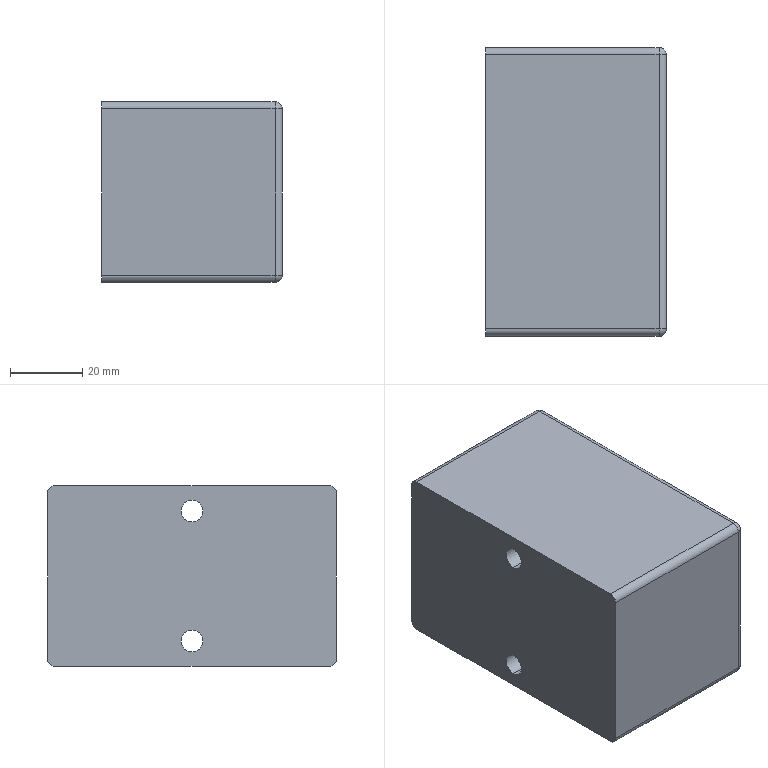Part | STEP file | 4-20.sldasm-Part-101 | 1 solid | 28 faces | box 50 x 80 x 50 mm | volume 195848 mm3 | cylinder 16 | plane 8 | sphere 4 | commonest cylinder face diameters 4 x8 6 x4 11 x4
STEP:
#1=CARTESIAN_POINT('',(268.,-172.617,-89.093));
#2=VERTEX_POINT('',#1);
#3=CARTESIAN_POINT('',(268.,-172.617,-78.093));
#4=VERTEX_POINT('',#3);
#5=CARTESIAN_POINT('',(268.,-172.617,-83.593));
#6=DIRECTION('',(1.,0.,0.));
#7=DIRECTION('',(0.,0.,-1.));
#8=AXIS2_PLACEMENT_3D('',#5,#6,#7);
#9=CIRCLE('',#8,5.5);
#10=EDGE_CURVE('',#2,#4,#9,.T.);
#11=ORIENTED_EDGE('',*,*,#10,.F.);
#12=CARTESIAN_POINT('',(274.936,-172.617,-89.093));
#13=VERTEX_POINT('',#12);
#14=CARTESIAN_POINT('',(268.,-172.617,-89.093));
#15=DIRECTION('',(1.,0.,0.));
#16=VECTOR('',#15,1000.);
#17=LINE('',#14,#16);
#18=EDGE_CURVE('',#2,#13,#17,.T.);
#19=ORIENTED_EDGE('',*,*,#18,.T.);
#20=CARTESIAN_POINT('',(275.,-170.326,-88.593));
#21=VERTEX_POINT('',#20);
#22=CARTESIAN_POINT('',(274.936,-172.617,-89.093));
#23=CARTESIAN_POINT('',(274.936,-172.225,-89.093));
#24=CARTESIAN_POINT('',(274.949,-171.836,-89.052));
#25=CARTESIAN_POINT('',(274.981,-171.063,-88.884));
#26=CARTESIAN_POINT('',(275.,-170.687,-88.758));
#27=CARTESIAN_POINT('',(275.,-170.326,-88.593));
#28=B_SPLINE_CURVE_WITH_KNOTS('',3,(#22,#23,#24,#25,#26,#27),.UNSPECIFIED.,.F.,.F.,(4,2,4),(0.002353,0.003528,0.004703),.UNSPECIFIED.);
#29=EDGE_CURVE('',#13,#21,#28,.T.);
#30=ORIENTED_EDGE('',*,*,#29,.T.);
#31=CARTESIAN_POINT('',(275.,-172.617,-78.093));
#32=VERTEX_POINT('',#31);
#33=CARTESIAN_POINT('',(275.,-172.617,-83.593));
#34=DIRECTION('',(1.,0.,0.));
#35=DIRECTION('',(0.,0.,-1.));
#36=AXIS2_PLACEMENT_3D('',#33,#34,#35);
#37=CIRCLE('',#36,5.5);
#38=EDGE_CURVE('',#21,#32,#37,.T.);
#39=ORIENTED_EDGE('',*,*,#38,.T.);
#40=CARTESIAN_POINT('',(268.,-172.617,-78.093));
#41=DIRECTION('',(1.,0.,0.));
#42=VECTOR('',#41,1000.);
#43=LINE('',#40,#42);
#44=EDGE_CURVE('',#4,#32,#43,.T.);
#45=ORIENTED_EDGE('',*,*,#44,.F.);
#46=EDGE_LOOP('',(#11,#19,#30,#39,#45));
#47=FACE_OUTER_BOUND('',#46,.T.);
#48=CARTESIAN_POINT('',(268.,-172.617,-83.593));
#49=DIRECTION('',(1.,0.,0.));
#50=DIRECTION('',(0.,0.,1.));
#51=AXIS2_PLACEMENT_3D('',#48,#49,#50);
#52=CYLINDRICAL_SURFACE('',#51,5.5);
#53=ADVANCED_FACE('',(#47),#52,.F.);
#54=CARTESIAN_POINT('',(268.,-172.617,-86.593));
#55=VERTEX_POINT('',#54);
#56=CARTESIAN_POINT('',(268.,-172.617,-80.593));
#57=VERTEX_POINT('',#56);
#58=CARTESIAN_POINT('',(268.,-172.617,-83.593));
#59=DIRECTION('',(1.,0.,0.));
#60=DIRECTION('',(0.,0.,-1.));
#61=AXIS2_PLACEMENT_3D('',#58,#59,#60);
#62=CIRCLE('',#61,3.);
#63=EDGE_CURVE('',#55,#57,#62,.T.);
#64=ORIENTED_EDGE('',*,*,#63,.T.);
#65=CARTESIAN_POINT('',(225.,-172.617,-80.593));
#66=VERTEX_POINT('',#65);
#67=CARTESIAN_POINT('',(232.,-172.617,-80.593));
#68=DIRECTION('',(-1.,0.,0.));
#69=VECTOR('',#68,1000.);
#70=LINE('',#67,#69);
#71=EDGE_CURVE('',#57,#66,#70,.T.);
#72=ORIENTED_EDGE('',*,*,#71,.T.);
#73=CARTESIAN_POINT('',(225.,-172.617,-86.593));
#74=VERTEX_POINT('',#73);
#75=CARTESIAN_POINT('',(225.,-172.617,-83.593));
#76=DIRECTION('',(1.,0.,0.));
#77=DIRECTION('',(0.,0.,1.));
#78=AXIS2_PLACEMENT_3D('',#75,#76,#77);
#79=CIRCLE('',#78,3.);
#80=EDGE_CURVE('',#74,#66,#79,.T.);
#81=ORIENTED_EDGE('',*,*,#80,.F.);
#82=CARTESIAN_POINT('',(232.,-172.617,-86.593));
#83=DIRECTION('',(-1.,0.,0.));
#84=VECTOR('',#83,1000.);
#85=LINE('',#82,#84);
#86=EDGE_CURVE('',#55,#74,#85,.T.);
#87=ORIENTED_EDGE('',*,*,#86,.F.);
#88=EDGE_LOOP('',(#64,#72,#81,#87));
#89=FACE_OUTER_BOUND('',#88,.T.);
#90=CARTESIAN_POINT('',(232.,-172.617,-83.593));
#91=DIRECTION('',(-1.,0.,0.));
#92=DIRECTION('',(0.,0.,-1.));
#93=AXIS2_PLACEMENT_3D('',#90,#91,#92);
#94=CYLINDRICAL_SURFACE('',#93,3.);
#95=ADVANCED_FACE('',(#89),#94,.F.);
#96=CARTESIAN_POINT('',(268.,-172.617,-53.093));
#97=VERTEX_POINT('',#96);
#98=CARTESIAN_POINT('',(268.,-172.617,-42.093));
#99=VERTEX_POINT('',#98);
#100=CARTESIAN_POINT('',(268.,-172.617,-47.593));
#101=DIRECTION('',(-1.,0.,0.));
#102=DIRECTION('',(0.,0.,1.));
#103=AXIS2_PLACEMENT_3D('',#100,#101,#102);
#104=CIRCLE('',#103,5.5);
#105=EDGE_CURVE('',#97,#99,#104,.T.);
#106=ORIENTED_EDGE('',*,*,#105,.T.);
#107=CARTESIAN_POINT('',(274.936,-172.617,-42.093));
#108=VERTEX_POINT('',#107);
#109=CARTESIAN_POINT('',(268.,-172.617,-42.093));
#110=DIRECTION('',(1.,0.,0.));
#111=VECTOR('',#110,1000.);
#112=LINE('',#109,#111);
#113=EDGE_CURVE('',#99,#108,#112,.T.);
#114=ORIENTED_EDGE('',*,*,#113,.T.);
#115=CARTESIAN_POINT('',(275.,-174.908,-42.593));
#116=VERTEX_POINT('',#115);
#117=CARTESIAN_POINT('',(274.936,-172.617,-42.093));
#118=CARTESIAN_POINT('',(274.936,-173.009,-42.093));
#119=CARTESIAN_POINT('',(274.949,-173.398,-42.134));
#120=CARTESIAN_POINT('',(274.981,-174.171,-42.302));
#121=CARTESIAN_POINT('',(275.,-174.547,-42.428));
#122=CARTESIAN_POINT('',(275.,-174.908,-42.593));
#123=B_SPLINE_CURVE_WITH_KNOTS('',3,(#117,#118,#119,#120,#121,#122),.UNSPECIFIED.,.F.,.F.,(4,2,4),(0.002353,0.003528,0.004703),.UNSPECIFIED.);
#124=EDGE_CURVE('',#108,#116,#123,.T.);
#125=ORIENTED_EDGE('',*,*,#124,.T.);
#126=CARTESIAN_POINT('',(275.,-172.617,-53.093));
#127=VERTEX_POINT('',#126);
#128=CARTESIAN_POINT('',(275.,-172.617,-47.593));
#129=DIRECTION('',(1.,0.,0.));
#130=DIRECTION('',(0.,0.,-1.));
#131=AXIS2_PLACEMENT_3D('',#128,#129,#130);
#132=CIRCLE('',#131,5.5);
#133=EDGE_CURVE('',#116,#127,#132,.T.);
#134=ORIENTED_EDGE('',*,*,#133,.T.);
#135=CARTESIAN_POINT('',(268.,-172.617,-53.093));
#136=DIRECTION('',(1.,0.,0.));
#137=VECTOR('',#136,1000.);
#138=LINE('',#135,#137);
#139=EDGE_CURVE('',#97,#127,#138,.T.);
#140=ORIENTED_EDGE('',*,*,#139,.F.);
#141=EDGE_LOOP('',(#106,#114,#125,#134,#140));
#142=FACE_OUTER_BOUND('',#141,.T.);
#143=CARTESIAN_POINT('',(268.,-172.617,-47.593));
#144=DIRECTION('',(1.,0.,0.));
#145=DIRECTION('',(0.,0.,-1.));
#146=AXIS2_PLACEMENT_3D('',#143,#144,#145);
#147=CYLINDRICAL_SURFACE('',#146,5.5);
#148=ADVANCED_FACE('',(#142),#147,.F.);
#149=CARTESIAN_POINT('',(268.,-172.617,-50.593));
#150=VERTEX_POINT('',#149);
#151=CARTESIAN_POINT('',(268.,-172.617,-44.593));
#152=VERTEX_POINT('',#151);
#153=CARTESIAN_POINT('',(268.,-172.617,-47.593));
#154=DIRECTION('',(-1.,0.,0.));
#155=DIRECTION('',(0.,0.,1.));
#156=AXIS2_PLACEMENT_3D('',#153,#154,#155);
#157=CIRCLE('',#156,3.);
#158=EDGE_CURVE('',#150,#152,#157,.T.);
#159=ORIENTED_EDGE('',*,*,#158,.F.);
#160=CARTESIAN_POINT('',(225.,-172.617,-50.593));
#161=VERTEX_POINT('',#160);
#162=CARTESIAN_POINT('',(232.,-172.617,-50.593));
#163=DIRECTION('',(-1.,0.,0.));
#164=VECTOR('',#163,1000.);
#165=LINE('',#162,#164);
#166=EDGE_CURVE('',#150,#161,#165,.T.);
#167=ORIENTED_EDGE('',*,*,#166,.T.);
#168=CARTESIAN_POINT('',(225.,-172.617,-44.593));
#169=VERTEX_POINT('',#168);
#170=CARTESIAN_POINT('',(225.,-172.617,-47.593));
#171=DIRECTION('',(1.,0.,0.));
#172=DIRECTION('',(0.,0.,1.));
#173=AXIS2_PLACEMENT_3D('',#170,#171,#172);
#174=CIRCLE('',#173,3.);
#175=EDGE_CURVE('',#169,#161,#174,.T.);
#176=ORIENTED_EDGE('',*,*,#175,.F.);
#177=CARTESIAN_POINT('',(232.,-172.617,-44.593));
#178=DIRECTION('',(-1.,0.,0.));
#179=VECTOR('',#178,1000.);
#180=LINE('',#177,#179);
#181=EDGE_CURVE('',#152,#169,#180,.T.);
#182=ORIENTED_EDGE('',*,*,#181,.F.);
#183=EDGE_LOOP('',(#159,#167,#176,#182));
#184=FACE_OUTER_BOUND('',#183,.T.);
#185=CARTESIAN_POINT('',(232.,-172.617,-47.593));
#186=DIRECTION('',(-1.,0.,0.));
#187=DIRECTION('',(0.,0.,1.));
#188=AXIS2_PLACEMENT_3D('',#185,#186,#187);
#189=CYLINDRICAL_SURFACE('',#188,3.);
#190=ADVANCED_FACE('',(#184),#189,.F.);
#191=ORIENTED_EDGE('',*,*,#175,.T.);
#192=CARTESIAN_POINT('',(225.,-172.617,-47.593));
#193=DIRECTION('',(1.,0.,0.));
#194=DIRECTION('',(0.,0.,1.));
#195=AXIS2_PLACEMENT_3D('',#192,#193,#194);
#196=CIRCLE('',#195,3.);
#197=EDGE_CURVE('',#161,#169,#196,.T.);
#198=ORIENTED_EDGE('',*,*,#197,.T.);
#199=EDGE_LOOP('',(#191,#198));
#200=FACE_BOUND('',#199,.T.);
#201=CARTESIAN_POINT('',(225.,-134.617,-90.593));
#202=VERTEX_POINT('',#201);
#203=CARTESIAN_POINT('',(225.,-210.617,-90.593));
#204=VERTEX_POINT('',#203);
#205=CARTESIAN_POINT('',(225.,-112.617,-90.593));
#206=DIRECTION('',(0.,-1.,0.));
#207=VECTOR('',#206,1000.);
#208=LINE('',#205,#207);
#209=EDGE_CURVE('',#202,#204,#208,.T.);
#210=ORIENTED_EDGE('',*,*,#209,.T.);
#211=CARTESIAN_POINT('',(225.,-212.617,-88.593));
#212=VERTEX_POINT('',#211);
#213=CARTESIAN_POINT('',(225.,-210.617,-88.593));
#214=DIRECTION('',(-1.,0.,0.));
#215=DIRECTION('',(0.,0.,1.));
#216=AXIS2_PLACEMENT_3D('',#213,#214,#215);
#217=CIRCLE('',#216,2.);
#218=EDGE_CURVE('',#204,#212,#217,.T.);
#219=ORIENTED_EDGE('',*,*,#218,.T.);
#220=CARTESIAN_POINT('',(225.,-212.617,-42.593));
#221=VERTEX_POINT('',#220);
#222=CARTESIAN_POINT('',(225.,-212.617,-65.593));
#223=DIRECTION('',(0.,0.,1.));
#224=VECTOR('',#223,1000.);
#225=LINE('',#222,#224);
#226=EDGE_CURVE('',#212,#221,#225,.T.);
#227=ORIENTED_EDGE('',*,*,#226,.T.);
#228=CARTESIAN_POINT('',(225.,-210.617,-40.593));
#229=VERTEX_POINT('',#228);
#230=CARTESIAN_POINT('',(225.,-210.617,-42.593));
#231=DIRECTION('',(-1.,0.,0.));
#232=DIRECTION('',(0.,0.,1.));
#233=AXIS2_PLACEMENT_3D('',#230,#231,#232);
#234=CIRCLE('',#233,2.);
#235=EDGE_CURVE('',#221,#229,#234,.T.);
#236=ORIENTED_EDGE('',*,*,#235,.T.);
#237=CARTESIAN_POINT('',(225.,-134.617,-40.593));
#238=VERTEX_POINT('',#237);
#239=CARTESIAN_POINT('',(225.,-112.617,-40.593));
#240=DIRECTION('',(0.,-1.,0.));
#241=VECTOR('',#240,1000.);
#242=LINE('',#239,#241);
#243=EDGE_CURVE('',#238,#229,#242,.T.);
#244=ORIENTED_EDGE('',*,*,#243,.F.);
#245=CARTESIAN_POINT('',(225.,-132.617,-42.593));
#246=VERTEX_POINT('',#245);
#247=CARTESIAN_POINT('',(225.,-134.617,-42.593));
#248=DIRECTION('',(-1.,0.,0.));
#249=DIRECTION('',(0.,0.,1.));
#250=AXIS2_PLACEMENT_3D('',#247,#248,#249);
#251=CIRCLE('',#250,2.);
#252=EDGE_CURVE('',#238,#246,#251,.T.);
#253=ORIENTED_EDGE('',*,*,#252,.T.);
#254=CARTESIAN_POINT('',(225.,-132.617,-88.593));
#255=VERTEX_POINT('',#254);
#256=CARTESIAN_POINT('',(225.,-132.617,-65.593));
#257=DIRECTION('',(0.,0.,-1.));
#258=VECTOR('',#257,1000.);
#259=LINE('',#256,#258);
#260=EDGE_CURVE('',#246,#255,#259,.T.);
#261=ORIENTED_EDGE('',*,*,#260,.T.);
#262=CARTESIAN_POINT('',(225.,-134.617,-88.593));
#263=DIRECTION('',(-1.,0.,0.));
#264=DIRECTION('',(0.,0.,1.));
#265=AXIS2_PLACEMENT_3D('',#262,#263,#264);
#266=CIRCLE('',#265,2.);
#267=EDGE_CURVE('',#255,#202,#266,.T.);
#268=ORIENTED_EDGE('',*,*,#267,.T.);
#269=EDGE_LOOP('',(#210,#219,#227,#236,#244,#253,#261,#268));
#270=FACE_OUTER_BOUND('',#269,.T.);
#271=ORIENTED_EDGE('',*,*,#80,.T.);
#272=CARTESIAN_POINT('',(225.,-172.617,-83.593));
#273=DIRECTION('',(1.,0.,0.));
#274=DIRECTION('',(0.,0.,1.));
#275=AXIS2_PLACEMENT_3D('',#272,#273,#274);
#276=CIRCLE('',#275,3.);
#277=EDGE_CURVE('',#66,#74,#276,.T.);
#278=ORIENTED_EDGE('',*,*,#277,.T.);
#279=EDGE_LOOP('',(#271,#278));
#280=FACE_BOUND('',#279,.T.);
#281=CARTESIAN_POINT('',(225.,-112.617,-65.593));
#282=DIRECTION('',(-1.,0.,0.));
#283=DIRECTION('',(0.,-1.,0.));
#284=AXIS2_PLACEMENT_3D('',#281,#282,#283);
#285=PLANE('',#284);
#286=ADVANCED_FACE('',(#200,#270,#280),#285,.T.);
#287=ORIENTED_EDGE('',*,*,#226,.F.);
#288=CARTESIAN_POINT('',(273.,-212.617,-88.593));
#289=VERTEX_POINT('',#288);
#290=CARTESIAN_POINT('',(250.,-212.617,-88.593));
#291=DIRECTION('',(1.,0.,0.));
#292=VECTOR('',#291,1000.);
#293=LINE('',#290,#292);
#294=EDGE_CURVE('',#212,#289,#293,.T.);
#295=ORIENTED_EDGE('',*,*,#294,.T.);
#296=CARTESIAN_POINT('',(273.,-212.617,-42.593));
#297=VERTEX_POINT('',#296);
#298=CARTESIAN_POINT('',(273.,-212.617,-65.593));
#299=DIRECTION('',(0.,0.,1.));
#300=VECTOR('',#299,1000.);
#301=LINE('',#298,#300);
#302=EDGE_CURVE('',#289,#297,#301,.T.);
#303=ORIENTED_EDGE('',*,*,#302,.T.);
#304=CARTESIAN_POINT('',(250.,-212.617,-42.593));
#305=DIRECTION('',(-1.,0.,0.));
#306=VECTOR('',#305,1000.);
#307=LINE('',#304,#306);
#308=EDGE_CURVE('',#297,#221,#307,.T.);
#309=ORIENTED_EDGE('',*,*,#308,.T.);
#310=EDGE_LOOP('',(#287,#295,#303,#309));
#311=FACE_OUTER_BOUND('',#310,.T.);
#312=CARTESIAN_POINT('',(250.,-212.617,-65.593));
#313=DIRECTION('',(0.,-1.,0.));
#314=DIRECTION('',(1.,0.,0.));
#315=AXIS2_PLACEMENT_3D('',#312,#313,#314);
#316=PLANE('',#315);
#317=ADVANCED_FACE('',(#311),#316,.T.);
#318=CARTESIAN_POINT('',(273.,-134.617,-90.593));
#319=VERTEX_POINT('',#318);
#320=CARTESIAN_POINT('',(273.,-210.617,-90.593));
#321=VERTEX_POINT('',#320);
#322=CARTESIAN_POINT('',(273.,-112.617,-90.593));
#323=DIRECTION('',(0.,-1.,0.));
#324=VECTOR('',#323,1000.);
#325=LINE('',#322,#324);
#326=EDGE_CURVE('',#319,#321,#325,.T.);
#327=ORIENTED_EDGE('',*,*,#326,.T.);
#328=CARTESIAN_POINT('',(250.,-210.617,-90.593));
#329=DIRECTION('',(-1.,0.,0.));
#330=VECTOR('',#329,1000.);
#331=LINE('',#328,#330);
#332=EDGE_CURVE('',#321,#204,#331,.T.);
#333=ORIENTED_EDGE('',*,*,#332,.T.);
#334=ORIENTED_EDGE('',*,*,#209,.F.);
#335=CARTESIAN_POINT('',(250.,-134.617,-90.593));
#336=DIRECTION('',(1.,0.,0.));
#337=VECTOR('',#336,1000.);
#338=LINE('',#335,#337);
#339=EDGE_CURVE('',#202,#319,#338,.T.);
#340=ORIENTED_EDGE('',*,*,#339,.T.);
#341=EDGE_LOOP('',(#327,#333,#334,#340));
#342=FACE_OUTER_BOUND('',#341,.T.);
#343=CARTESIAN_POINT('',(250.,-112.617,-90.593));
#344=DIRECTION('',(0.,0.,-1.));
#345=DIRECTION('',(0.,1.,0.));
#346=AXIS2_PLACEMENT_3D('',#343,#344,#345);
#347=PLANE('',#346);
#348=ADVANCED_FACE('',(#342),#347,.T.);
#349=CARTESIAN_POINT('',(273.,-210.617,-40.593));
#350=VERTEX_POINT('',#349);
#351=CARTESIAN_POINT('',(273.,-134.617,-40.593));
#352=VERTEX_POINT('',#351);
#353=CARTESIAN_POINT('',(273.,-112.617,-40.593));
#354=DIRECTION('',(0.,1.,0.));
#355=VECTOR('',#354,1000.);
#356=LINE('',#353,#355);
#357=EDGE_CURVE('',#350,#352,#356,.T.);
#358=ORIENTED_EDGE('',*,*,#357,.T.);
#359=CARTESIAN_POINT('',(250.,-134.617,-40.593));
#360=DIRECTION('',(-1.,0.,0.));
#361=VECTOR('',#360,1000.);
#362=LINE('',#359,#361);
#363=EDGE_CURVE('',#352,#238,#362,.T.);
#364=ORIENTED_EDGE('',*,*,#363,.T.);
#365=ORIENTED_EDGE('',*,*,#243,.T.);
#366=CARTESIAN_POINT('',(250.,-210.617,-40.593));
#367=DIRECTION('',(1.,0.,0.));
#368=VECTOR('',#367,1000.);
#369=LINE('',#366,#368);
#370=EDGE_CURVE('',#229,#350,#369,.T.);
#371=ORIENTED_EDGE('',*,*,#370,.T.);
#372=EDGE_LOOP('',(#358,#364,#365,#371));
#373=FACE_OUTER_BOUND('',#372,.T.);
#374=CARTESIAN_POINT('',(250.,-112.617,-40.593));
#375=DIRECTION('',(0.,0.,1.));
#376=DIRECTION('',(0.,-1.,0.));
#377=AXIS2_PLACEMENT_3D('',#374,#375,#376);
#378=PLANE('',#377);
#379=ADVANCED_FACE('',(#373),#378,.T.);
#380=CARTESIAN_POINT('',(273.,-132.617,-42.593));
#381=VERTEX_POINT('',#380);
#382=CARTESIAN_POINT('',(273.,-132.617,-88.593));
#383=VERTEX_POINT('',#382);
#384=CARTESIAN_POINT('',(273.,-132.617,-65.593));
#385=DIRECTION('',(0.,0.,-1.));
#386=VECTOR('',#385,1000.);
#387=LINE('',#384,#386);
#388=EDGE_CURVE('',#381,#383,#387,.T.);
#389=ORIENTED_EDGE('',*,*,#388,.T.);
#390=CARTESIAN_POINT('',(250.,-132.617,-88.593));
#391=DIRECTION('',(-1.,0.,0.));
#392=VECTOR('',#391,1000.);
#393=LINE('',#390,#392);
#394=EDGE_CURVE('',#383,#255,#393,.T.);
#395=ORIENTED_EDGE('',*,*,#394,.T.);
#396=ORIENTED_EDGE('',*,*,#260,.F.);
#397=CARTESIAN_POINT('',(250.,-132.617,-42.593));
#398=DIRECTION('',(1.,0.,0.));
#399=VECTOR('',#398,1000.);
#400=LINE('',#397,#399);
#401=EDGE_CURVE('',#246,#381,#400,.T.);
#402=ORIENTED_EDGE('',*,*,#401,.T.);
#403=EDGE_LOOP('',(#389,#395,#396,#402));
#404=FACE_OUTER_BOUND('',#403,.T.);
#405=CARTESIAN_POINT('',(250.,-132.617,-65.593));
#406=DIRECTION('',(0.,1.,0.));
#407=DIRECTION('',(-1.,0.,0.));
#408=AXIS2_PLACEMENT_3D('',#405,#406,#407);
#409=PLANE('',#408);
#410=ADVANCED_FACE('',(#404),#409,.T.);
#411=ORIENTED_EDGE('',*,*,#38,.F.);
#412=CARTESIAN_POINT('',(275.,-134.617,-88.593));
#413=VERTEX_POINT('',#412);
#414=CARTESIAN_POINT('',(275.,-112.617,-88.593));
#415=DIRECTION('',(0.,1.,0.));
#416=VECTOR('',#415,1000.);
#417=LINE('',#414,#416);
#418=EDGE_CURVE('',#21,#413,#417,.T.);
#419=ORIENTED_EDGE('',*,*,#418,.T.);
#420=CARTESIAN_POINT('',(275.,-134.617,-42.593));
#421=VERTEX_POINT('',#420);
#422=CARTESIAN_POINT('',(275.,-134.617,-65.593));
#423=DIRECTION('',(0.,0.,1.));
#424=VECTOR('',#423,1000.);
#425=LINE('',#422,#424);
#426=EDGE_CURVE('',#413,#421,#425,.T.);
#427=ORIENTED_EDGE('',*,*,#426,.T.);
#428=CARTESIAN_POINT('',(275.,-170.326,-42.593));
#429=VERTEX_POINT('',#428);
#430=CARTESIAN_POINT('',(275.,-112.617,-42.593));
#431=DIRECTION('',(0.,-1.,0.));
#432=VECTOR('',#431,1000.);
#433=LINE('',#430,#432);
#434=EDGE_CURVE('',#421,#429,#433,.T.);
#435=ORIENTED_EDGE('',*,*,#434,.T.);
#436=CARTESIAN_POINT('',(275.,-172.617,-47.593));
#437=DIRECTION('',(1.,0.,0.));
#438=DIRECTION('',(0.,0.,-1.));
#439=AXIS2_PLACEMENT_3D('',#436,#437,#438);
#440=CIRCLE('',#439,5.5);
#441=EDGE_CURVE('',#127,#429,#440,.T.);
#442=ORIENTED_EDGE('',*,*,#441,.F.);
#443=ORIENTED_EDGE('',*,*,#133,.F.);
#444=CARTESIAN_POINT('',(275.,-210.617,-42.593));
#445=VERTEX_POINT('',#444);
#446=CARTESIAN_POINT('',(275.,-112.617,-42.593));
#447=DIRECTION('',(0.,-1.,0.));
#448=VECTOR('',#447,1000.);
#449=LINE('',#446,#448);
#450=EDGE_CURVE('',#116,#445,#449,.T.);
#451=ORIENTED_EDGE('',*,*,#450,.T.);
#452=CARTESIAN_POINT('',(275.,-210.617,-88.593));
#453=VERTEX_POINT('',#452);
#454=CARTESIAN_POINT('',(275.,-210.617,-65.593));
#455=DIRECTION('',(0.,0.,-1.));
#456=VECTOR('',#455,1000.);
#457=LINE('',#454,#456);
#458=EDGE_CURVE('',#445,#453,#457,.T.);
#459=ORIENTED_EDGE('',*,*,#458,.T.);
#460=CARTESIAN_POINT('',(275.,-174.908,-88.593));
#461=VERTEX_POINT('',#460);
#462=CARTESIAN_POINT('',(275.,-112.617,-88.593));
#463=DIRECTION('',(0.,1.,0.));
#464=VECTOR('',#463,1000.);
#465=LINE('',#462,#464);
#466=EDGE_CURVE('',#453,#461,#465,.T.);
#467=ORIENTED_EDGE('',*,*,#466,.T.);
#468=CARTESIAN_POINT('',(275.,-172.617,-83.593));
#469=DIRECTION('',(1.,0.,0.));
#470=DIRECTION('',(0.,0.,-1.));
#471=AXIS2_PLACEMENT_3D('',#468,#469,#470);
#472=CIRCLE('',#471,5.5);
#473=EDGE_CURVE('',#32,#461,#472,.T.);
#474=ORIENTED_EDGE('',*,*,#473,.F.);
#475=EDGE_LOOP('',(#411,#419,#427,#435,#442,#443,#451,#459,#467,#474));
#476=FACE_OUTER_BOUND('',#475,.T.);
#477=CARTESIAN_POINT('',(275.,-112.617,-65.593));
#478=DIRECTION('',(1.,0.,0.));
#479=DIRECTION('',(0.,1.,0.));
#480=AXIS2_PLACEMENT_3D('',#477,#478,#479);
#481=PLANE('',#480);
#482=ADVANCED_FACE('',(#476),#481,.T.);
#483=ORIENTED_EDGE('',*,*,#166,.F.);
#484=CARTESIAN_POINT('',(268.,-172.617,-47.593));
#485=DIRECTION('',(-1.,0.,0.));
#486=DIRECTION('',(0.,0.,1.));
#487=AXIS2_PLACEMENT_3D('',#484,#485,#486);
#488=CIRCLE('',#487,3.);
#489=EDGE_CURVE('',#152,#150,#488,.T.);
#490=ORIENTED_EDGE('',*,*,#489,.F.);
#491=ORIENTED_EDGE('',*,*,#181,.T.);
#492=ORIENTED_EDGE('',*,*,#197,.F.);
#493=EDGE_LOOP('',(#483,#490,#491,#492));
#494=FACE_OUTER_BOUND('',#493,.T.);
#495=CARTESIAN_POINT('',(232.,-172.617,-47.593));
#496=DIRECTION('',(-1.,0.,0.));
#497=DIRECTION('',(0.,0.,1.));
#498=AXIS2_PLACEMENT_3D('',#495,#496,#497);
#499=CYLINDRICAL_SURFACE('',#498,3.);
#500=ADVANCED_FACE('',(#494),#499,.F.);
#501=ORIENTED_EDGE('',*,*,#105,.F.);
#502=CARTESIAN_POINT('',(268.,-172.617,-47.593));
#503=DIRECTION('',(-1.,0.,0.));
#504=DIRECTION('',(0.,0.,1.));
#505=AXIS2_PLACEMENT_3D('',#502,#503,#504);
#506=CIRCLE('',#505,5.5);
#507=EDGE_CURVE('',#99,#97,#506,.T.);
#508=ORIENTED_EDGE('',*,*,#507,.F.);
#509=EDGE_LOOP('',(#501,#508));
#510=FACE_OUTER_BOUND('',#509,.T.);
#511=ORIENTED_EDGE('',*,*,#489,.T.);
#512=ORIENTED_EDGE('',*,*,#158,.T.);
#513=EDGE_LOOP('',(#511,#512));
#514=FACE_BOUND('',#513,.T.);
#515=CARTESIAN_POINT('',(268.,-172.617,-47.593));
#516=DIRECTION('',(-1.,0.,0.));
#517=DIRECTION('',(0.,0.,1.));
#518=AXIS2_PLACEMENT_3D('',#515,#516,#517);
#519=PLANE('',#518);
#520=ADVANCED_FACE('',(#510,#514),#519,.F.);
#521=ORIENTED_EDGE('',*,*,#113,.F.);
#522=ORIENTED_EDGE('',*,*,#507,.T.);
#523=ORIENTED_EDGE('',*,*,#139,.T.);
#524=ORIENTED_EDGE('',*,*,#441,.T.);
#525=CARTESIAN_POINT('',(275.,-170.326,-42.593));
#526=CARTESIAN_POINT('',(275.,-170.687,-42.427));
#527=CARTESIAN_POINT('',(274.981,-171.059,-42.304));
#528=CARTESIAN_POINT('',(274.949,-171.826,-42.136));
#529=CARTESIAN_POINT('',(274.936,-172.224,-42.093));
#530=CARTESIAN_POINT('',(274.936,-172.617,-42.093));
#531=B_SPLINE_CURVE_WITH_KNOTS('',3,(#525,#526,#527,#528,#529,#530),.UNSPECIFIED.,.F.,.F.,(4,2,4),(0.,0.001176,0.002353),.UNSPECIFIED.);
#532=EDGE_CURVE('',#429,#108,#531,.T.);
#533=ORIENTED_EDGE('',*,*,#532,.T.);
#534=EDGE_LOOP('',(#521,#522,#523,#524,#533));
#535=FACE_OUTER_BOUND('',#534,.T.);
#536=CARTESIAN_POINT('',(268.,-172.617,-47.593));
#537=DIRECTION('',(1.,0.,0.));
#538=DIRECTION('',(0.,0.,-1.));
#539=AXIS2_PLACEMENT_3D('',#536,#537,#538);
#540=CYLINDRICAL_SURFACE('',#539,5.5);
#541=ADVANCED_FACE('',(#535),#540,.F.);
#542=ORIENTED_EDGE('',*,*,#71,.F.);
#543=CARTESIAN_POINT('',(268.,-172.617,-83.593));
#544=DIRECTION('',(1.,0.,0.));
#545=DIRECTION('',(0.,0.,-1.));
#546=AXIS2_PLACEMENT_3D('',#543,#544,#545);
#547=CIRCLE('',#546,3.);
#548=EDGE_CURVE('',#57,#55,#547,.T.);
#549=ORIENTED_EDGE('',*,*,#548,.T.);
#550=ORIENTED_EDGE('',*,*,#86,.T.);
#551=ORIENTED_EDGE('',*,*,#277,.F.);
#552=EDGE_LOOP('',(#542,#549,#550,#551));
#553=FACE_OUTER_BOUND('',#552,.T.);
#554=CARTESIAN_POINT('',(232.,-172.617,-83.593));
#555=DIRECTION('',(-1.,0.,0.));
#556=DIRECTION('',(0.,0.,-1.));
#557=AXIS2_PLACEMENT_3D('',#554,#555,#556);
#558=CYLINDRICAL_SURFACE('',#557,3.);
#559=ADVANCED_FACE('',(#553),#558,.F.);
#560=CARTESIAN_POINT('',(268.,-172.617,-83.593));
#561=DIRECTION('',(1.,0.,0.));
#562=DIRECTION('',(0.,0.,-1.));
#563=AXIS2_PLACEMENT_3D('',#560,#561,#562);
#564=CIRCLE('',#563,5.5);
#565=EDGE_CURVE('',#4,#2,#564,.T.);
#566=ORIENTED_EDGE('',*,*,#565,.T.);
#567=ORIENTED_EDGE('',*,*,#10,.T.);
#568=EDGE_LOOP('',(#566,#567));
#569=FACE_OUTER_BOUND('',#568,.T.);
#570=ORIENTED_EDGE('',*,*,#63,.F.);
#571=ORIENTED_EDGE('',*,*,#548,.F.);
#572=EDGE_LOOP('',(#570,#571));
#573=FACE_BOUND('',#572,.T.);
#574=CARTESIAN_POINT('',(268.,-172.617,-83.593));
#575=DIRECTION('',(-1.,0.,0.));
#576=DIRECTION('',(0.,0.,-1.));
#577=AXIS2_PLACEMENT_3D('',#574,#575,#576);
#578=PLANE('',#577);
#579=ADVANCED_FACE('',(#569,#573),#578,.F.);
#580=ORIENTED_EDGE('',*,*,#18,.F.);
#581=ORIENTED_EDGE('',*,*,#565,.F.);
#582=ORIENTED_EDGE('',*,*,#44,.T.);
#583=ORIENTED_EDGE('',*,*,#473,.T.);
#584=CARTESIAN_POINT('',(275.,-174.908,-88.593));
#585=CARTESIAN_POINT('',(275.,-174.547,-88.759));
#586=CARTESIAN_POINT('',(274.981,-174.174,-88.882));
#587=CARTESIAN_POINT('',(274.949,-173.408,-89.05));
#588=CARTESIAN_POINT('',(274.936,-173.009,-89.093));
#589=CARTESIAN_POINT('',(274.936,-172.617,-89.093));
#590=B_SPLINE_CURVE_WITH_KNOTS('',3,(#584,#585,#586,#587,#588,#589),.UNSPECIFIED.,.F.,.F.,(4,2,4),(0.,0.001176,0.002353),.UNSPECIFIED.);
#591=EDGE_CURVE('',#461,#13,#590,.T.);
#592=ORIENTED_EDGE('',*,*,#591,.T.);
#593=EDGE_LOOP('',(#580,#581,#582,#583,#592));
#594=FACE_OUTER_BOUND('',#593,.T.);
#595=CARTESIAN_POINT('',(268.,-172.617,-83.593));
#596=DIRECTION('',(1.,0.,0.));
#597=DIRECTION('',(0.,0.,1.));
#598=AXIS2_PLACEMENT_3D('',#595,#596,#597);
#599=CYLINDRICAL_SURFACE('',#598,5.5);
#600=ADVANCED_FACE('',(#594),#599,.F.);
#601=CARTESIAN_POINT('',(273.,-134.617,-42.593));
#602=DIRECTION('',(1.,0.,0.));
#603=DIRECTION('',(0.,0.,-1.));
#604=AXIS2_PLACEMENT_3D('',#601,#602,#603);
#605=CIRCLE('',#604,2.);
#606=EDGE_CURVE('',#381,#352,#605,.T.);
#607=ORIENTED_EDGE('',*,*,#606,.F.);
#608=ORIENTED_EDGE('',*,*,#401,.F.);
#609=ORIENTED_EDGE('',*,*,#252,.F.);
#610=ORIENTED_EDGE('',*,*,#363,.F.);
#611=EDGE_LOOP('',(#607,#608,#609,#610));
#612=FACE_OUTER_BOUND('',#611,.T.);
#613=CARTESIAN_POINT('',(250.,-134.617,-42.593));
#614=DIRECTION('',(-1.,0.,0.));
#615=DIRECTION('',(0.,0.,1.));
#616=AXIS2_PLACEMENT_3D('',#613,#614,#615);
#617=CYLINDRICAL_SURFACE('',#616,2.);
#618=ADVANCED_FACE('',(#612),#617,.T.);
#619=CARTESIAN_POINT('',(273.,-134.617,-42.593));
#620=DIRECTION('',(0.,0.,-1.));
#621=DIRECTION('',(1.,0.,0.));
#622=AXIS2_PLACEMENT_3D('',#619,#620,#621);
#623=CIRCLE('',#622,2.);
#624=EDGE_CURVE('',#381,#421,#623,.T.);
#625=ORIENTED_EDGE('',*,*,#624,.F.);
#626=ORIENTED_EDGE('',*,*,#606,.T.);
#627=CARTESIAN_POINT('',(273.,-134.617,-42.593));
#628=DIRECTION('',(0.,-1.,0.));
#629=DIRECTION('',(0.,0.,1.));
#630=AXIS2_PLACEMENT_3D('',#627,#628,#629);
#631=CIRCLE('',#630,2.);
#632=EDGE_CURVE('',#421,#352,#631,.T.);
#633=ORIENTED_EDGE('',*,*,#632,.F.);
#634=EDGE_LOOP('',(#625,#626,#633));
#635=FACE_OUTER_BOUND('',#634,.T.);
#636=CARTESIAN_POINT('',(273.,-134.617,-42.593));
#637=DIRECTION('',(0.,1.,0.));
#638=DIRECTION('',(1.,0.,0.));
#639=AXIS2_PLACEMENT_3D('',#636,#637,#638);
#640=SPHERICAL_SURFACE('',#639,2.);
#641=ADVANCED_FACE('',(#635),#640,.T.);
#642=ORIENTED_EDGE('',*,*,#235,.F.);
#643=ORIENTED_EDGE('',*,*,#308,.F.);
#644=CARTESIAN_POINT('',(273.,-210.617,-42.593));
#645=DIRECTION('',(1.,0.,0.));
#646=DIRECTION('',(0.,0.,-1.));
#647=AXIS2_PLACEMENT_3D('',#644,#645,#646);
#648=CIRCLE('',#647,2.);
#649=EDGE_CURVE('',#350,#297,#648,.T.);
#650=ORIENTED_EDGE('',*,*,#649,.F.);
#651=ORIENTED_EDGE('',*,*,#370,.F.);
#652=EDGE_LOOP('',(#642,#643,#650,#651));
#653=FACE_OUTER_BOUND('',#652,.T.);
#654=CARTESIAN_POINT('',(250.,-210.617,-42.593));
#655=DIRECTION('',(1.,0.,0.));
#656=DIRECTION('',(0.,0.,-1.));
#657=AXIS2_PLACEMENT_3D('',#654,#655,#656);
#658=CYLINDRICAL_SURFACE('',#657,2.);
#659=ADVANCED_FACE('',(#653),#658,.T.);
#660=ORIENTED_EDGE('',*,*,#632,.T.);
#661=ORIENTED_EDGE('',*,*,#357,.F.);
#662=CARTESIAN_POINT('',(273.,-210.617,-42.593));
#663=DIRECTION('',(0.,-1.,0.));
#664=DIRECTION('',(0.,0.,-1.));
#665=AXIS2_PLACEMENT_3D('',#662,#663,#664);
#666=CIRCLE('',#665,2.);
#667=EDGE_CURVE('',#445,#350,#666,.T.);
#668=ORIENTED_EDGE('',*,*,#667,.F.);
#669=ORIENTED_EDGE('',*,*,#450,.F.);
#670=ORIENTED_EDGE('',*,*,#124,.F.);
#671=ORIENTED_EDGE('',*,*,#532,.F.);
#672=ORIENTED_EDGE('',*,*,#434,.F.);
#673=EDGE_LOOP('',(#660,#661,#668,#669,#670,#671,#672));
#674=FACE_OUTER_BOUND('',#673,.T.);
#675=CARTESIAN_POINT('',(273.,-112.617,-42.593));
#676=DIRECTION('',(0.,-1.,0.));
#677=DIRECTION('',(0.,0.,-1.));
#678=AXIS2_PLACEMENT_3D('',#675,#676,#677);
#679=CYLINDRICAL_SURFACE('',#678,2.);
#680=ADVANCED_FACE('',(#674),#679,.T.);
#681=ORIENTED_EDGE('',*,*,#624,.T.);
#682=ORIENTED_EDGE('',*,*,#426,.F.);
#683=CARTESIAN_POINT('',(273.,-134.617,-88.593));
#684=DIRECTION('',(0.,0.,-1.));
#685=DIRECTION('',(-1.,0.,0.));
#686=AXIS2_PLACEMENT_3D('',#683,#684,#685);
#687=CIRCLE('',#686,2.);
#688=EDGE_CURVE('',#383,#413,#687,.T.);
#689=ORIENTED_EDGE('',*,*,#688,.F.);
#690=ORIENTED_EDGE('',*,*,#388,.F.);
#691=EDGE_LOOP('',(#681,#682,#689,#690));
#692=FACE_OUTER_BOUND('',#691,.T.);
#693=CARTESIAN_POINT('',(273.,-134.617,-65.593));
#694=DIRECTION('',(0.,0.,1.));
#695=DIRECTION('',(1.,0.,0.));
#696=AXIS2_PLACEMENT_3D('',#693,#694,#695);
#697=CYLINDRICAL_SURFACE('',#696,2.);
#698=ADVANCED_FACE('',(#692),#697,.T.);
#699=ORIENTED_EDGE('',*,*,#267,.F.);
#700=ORIENTED_EDGE('',*,*,#394,.F.);
#701=CARTESIAN_POINT('',(273.,-134.617,-88.593));
#702=DIRECTION('',(1.,0.,0.));
#703=DIRECTION('',(0.,0.,-1.));
#704=AXIS2_PLACEMENT_3D('',#701,#702,#703);
#705=CIRCLE('',#704,2.);
#706=EDGE_CURVE('',#319,#383,#705,.T.);
#707=ORIENTED_EDGE('',*,*,#706,.F.);
#708=ORIENTED_EDGE('',*,*,#339,.F.);
#709=EDGE_LOOP('',(#699,#700,#707,#708));
#710=FACE_OUTER_BOUND('',#709,.T.);
#711=CARTESIAN_POINT('',(250.,-134.617,-88.593));
#712=DIRECTION('',(1.,0.,0.));
#713=DIRECTION('',(0.,0.,-1.));
#714=AXIS2_PLACEMENT_3D('',#711,#712,#713);
#715=CYLINDRICAL_SURFACE('',#714,2.);
#716=ADVANCED_FACE('',(#710),#715,.T.);
#717=ORIENTED_EDGE('',*,*,#667,.T.);
#718=ORIENTED_EDGE('',*,*,#649,.T.);
#719=CARTESIAN_POINT('',(273.,-210.617,-42.593));
#720=DIRECTION('',(0.,0.,-1.));
#721=DIRECTION('',(1.,0.,0.));
#722=AXIS2_PLACEMENT_3D('',#719,#720,#721);
#723=CIRCLE('',#722,2.);
#724=EDGE_CURVE('',#445,#297,#723,.T.);
#725=ORIENTED_EDGE('',*,*,#724,.F.);
#726=EDGE_LOOP('',(#717,#718,#725));
#727=FACE_OUTER_BOUND('',#726,.T.);
#728=CARTESIAN_POINT('',(273.,-210.617,-42.593));
#729=DIRECTION('',(0.,1.,0.));
#730=DIRECTION('',(1.,0.,0.));
#731=AXIS2_PLACEMENT_3D('',#728,#729,#730);
#732=SPHERICAL_SURFACE('',#731,2.);
#733=ADVANCED_FACE('',(#727),#732,.T.);
#734=ORIENTED_EDGE('',*,*,#706,.T.);
#735=ORIENTED_EDGE('',*,*,#688,.T.);
#736=CARTESIAN_POINT('',(273.,-134.617,-88.593));
#737=DIRECTION('',(0.,-1.,0.));
#738=DIRECTION('',(0.,0.,1.));
#739=AXIS2_PLACEMENT_3D('',#736,#737,#738);
#740=CIRCLE('',#739,2.);
#741=EDGE_CURVE('',#319,#413,#740,.T.);
#742=ORIENTED_EDGE('',*,*,#741,.F.);
#743=EDGE_LOOP('',(#734,#735,#742));
#744=FACE_OUTER_BOUND('',#743,.T.);
#745=CARTESIAN_POINT('',(273.,-134.617,-88.593));
#746=DIRECTION('',(0.,1.,0.));
#747=DIRECTION('',(1.,0.,0.));
#748=AXIS2_PLACEMENT_3D('',#745,#746,#747);
#749=SPHERICAL_SURFACE('',#748,2.);
#750=ADVANCED_FACE('',(#744),#749,.T.);
#751=ORIENTED_EDGE('',*,*,#724,.T.);
#752=ORIENTED_EDGE('',*,*,#302,.F.);
#753=CARTESIAN_POINT('',(273.,-210.617,-88.593));
#754=DIRECTION('',(0.,0.,-1.));
#755=DIRECTION('',(-1.,0.,0.));
#756=AXIS2_PLACEMENT_3D('',#753,#754,#755);
#757=CIRCLE('',#756,2.);
#758=EDGE_CURVE('',#453,#289,#757,.T.);
#759=ORIENTED_EDGE('',*,*,#758,.F.);
#760=ORIENTED_EDGE('',*,*,#458,.F.);
#761=EDGE_LOOP('',(#751,#752,#759,#760));
#762=FACE_OUTER_BOUND('',#761,.T.);
#763=CARTESIAN_POINT('',(273.,-210.617,-65.593));
#764=DIRECTION('',(0.,0.,-1.));
#765=DIRECTION('',(-1.,0.,0.));
#766=AXIS2_PLACEMENT_3D('',#763,#764,#765);
#767=CYLINDRICAL_SURFACE('',#766,2.);
#768=ADVANCED_FACE('',(#762),#767,.T.);
#769=ORIENTED_EDGE('',*,*,#591,.F.);
#770=ORIENTED_EDGE('',*,*,#466,.F.);
#771=CARTESIAN_POINT('',(273.,-210.617,-88.593));
#772=DIRECTION('',(0.,-1.,0.));
#773=DIRECTION('',(0.,0.,-1.));
#774=AXIS2_PLACEMENT_3D('',#771,#772,#773);
#775=CIRCLE('',#774,2.);
#776=EDGE_CURVE('',#321,#453,#775,.T.);
#777=ORIENTED_EDGE('',*,*,#776,.F.);
#778=ORIENTED_EDGE('',*,*,#326,.F.);
#779=ORIENTED_EDGE('',*,*,#741,.T.);
#780=ORIENTED_EDGE('',*,*,#418,.F.);
#781=ORIENTED_EDGE('',*,*,#29,.F.);
#782=EDGE_LOOP('',(#769,#770,#777,#778,#779,#780,#781));
#783=FACE_OUTER_BOUND('',#782,.T.);
#784=CARTESIAN_POINT('',(273.,-112.617,-88.593));
#785=DIRECTION('',(0.,-1.,0.));
#786=DIRECTION('',(0.,0.,-1.));
#787=AXIS2_PLACEMENT_3D('',#784,#785,#786);
#788=CYLINDRICAL_SURFACE('',#787,2.);
#789=ADVANCED_FACE('',(#783),#788,.T.);
#790=ORIENTED_EDGE('',*,*,#776,.T.);
#791=ORIENTED_EDGE('',*,*,#758,.T.);
#792=CARTESIAN_POINT('',(273.,-210.617,-88.593));
#793=DIRECTION('',(-1.,0.,0.));
#794=DIRECTION('',(0.,0.,-1.));
#795=AXIS2_PLACEMENT_3D('',#792,#793,#794);
#796=CIRCLE('',#795,2.);
#797=EDGE_CURVE('',#321,#289,#796,.T.);
#798=ORIENTED_EDGE('',*,*,#797,.F.);
#799=EDGE_LOOP('',(#790,#791,#798));
#800=FACE_OUTER_BOUND('',#799,.T.);
#801=CARTESIAN_POINT('',(273.,-210.617,-88.593));
#802=DIRECTION('',(0.,1.,0.));
#803=DIRECTION('',(1.,0.,0.));
#804=AXIS2_PLACEMENT_3D('',#801,#802,#803);
#805=SPHERICAL_SURFACE('',#804,2.);
#806=ADVANCED_FACE('',(#800),#805,.T.);
#807=ORIENTED_EDGE('',*,*,#797,.T.);
#808=ORIENTED_EDGE('',*,*,#294,.F.);
#809=ORIENTED_EDGE('',*,*,#218,.F.);
#810=ORIENTED_EDGE('',*,*,#332,.F.);
#811=EDGE_LOOP('',(#807,#808,#809,#810));
#812=FACE_OUTER_BOUND('',#811,.T.);
#813=CARTESIAN_POINT('',(250.,-210.617,-88.593));
#814=DIRECTION('',(-1.,0.,0.));
#815=DIRECTION('',(0.,0.,1.));
#816=AXIS2_PLACEMENT_3D('',#813,#814,#815);
#817=CYLINDRICAL_SURFACE('',#816,2.);
#818=ADVANCED_FACE('',(#812),#817,.T.);
#819=CLOSED_SHELL('',(#53,#95,#148,#190,#286,#317,#348,#379,#410,#482,#500,#520,#541,#559,#579,#600,#618,#641,#659,#680,#698,#716,#733,#750,#768,#789,#806,#818));
#820=MANIFOLD_SOLID_BREP('',#819);
#821=CARTESIAN_POINT('',(0.,0.,0.));
#822=DIRECTION('',(0.,0.,1.));
#823=DIRECTION('',(1.,0.,0.));
#824=AXIS2_PLACEMENT_3D('',#821,#822,#823);
#825=(LENGTH_UNIT()NAMED_UNIT(*)SI_UNIT(.MILLI.,.METRE.));
#826=UNCERTAINTY_MEASURE_WITH_UNIT(LENGTH_MEASURE(0.00001),#825,'','');
#827=(NAMED_UNIT(*)PLANE_ANGLE_UNIT()SI_UNIT($,.RADIAN.));
#828=(NAMED_UNIT(*)SI_UNIT($,.STERADIAN.)SOLID_ANGLE_UNIT());
#829=(GEOMETRIC_REPRESENTATION_CONTEXT(3)GLOBAL_UNCERTAINTY_ASSIGNED_CONTEXT((#826))GLOBAL_UNIT_ASSIGNED_CONTEXT((#825,#827,#828))REPRESENTATION_CONTEXT('',''));
#830=ADVANCED_BREP_SHAPE_REPRESENTATION('',(#820,#824),#829);